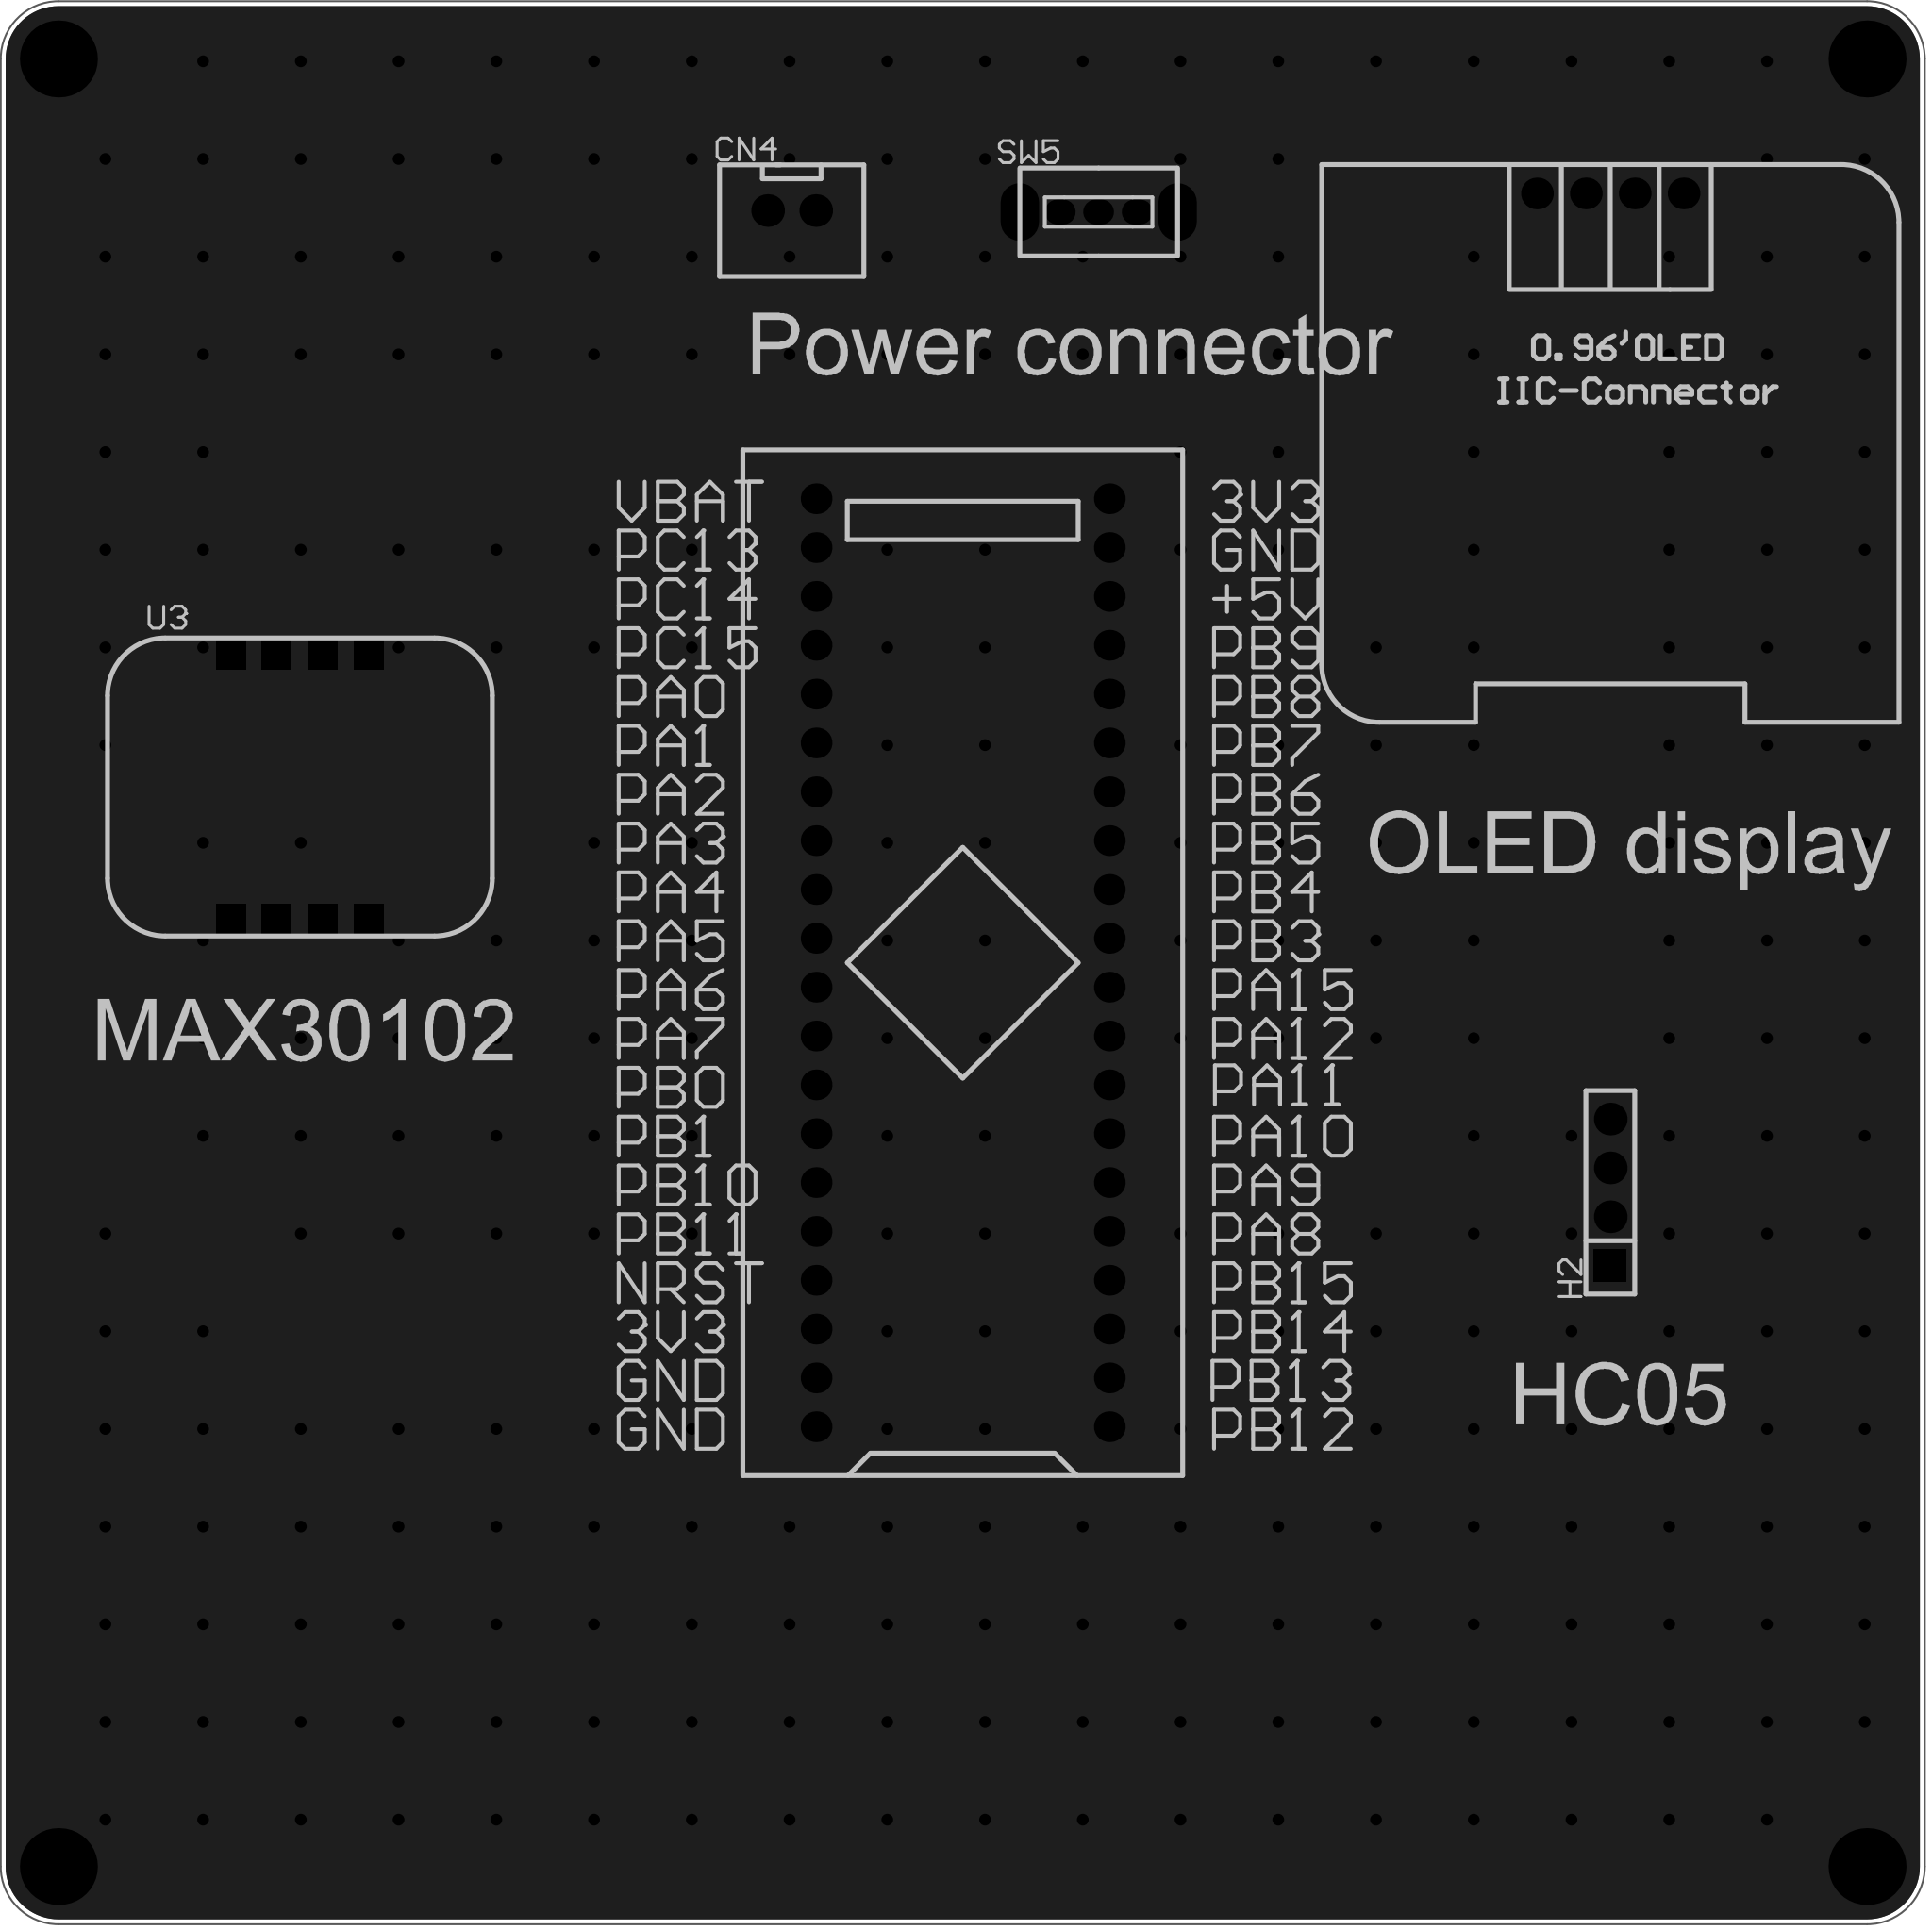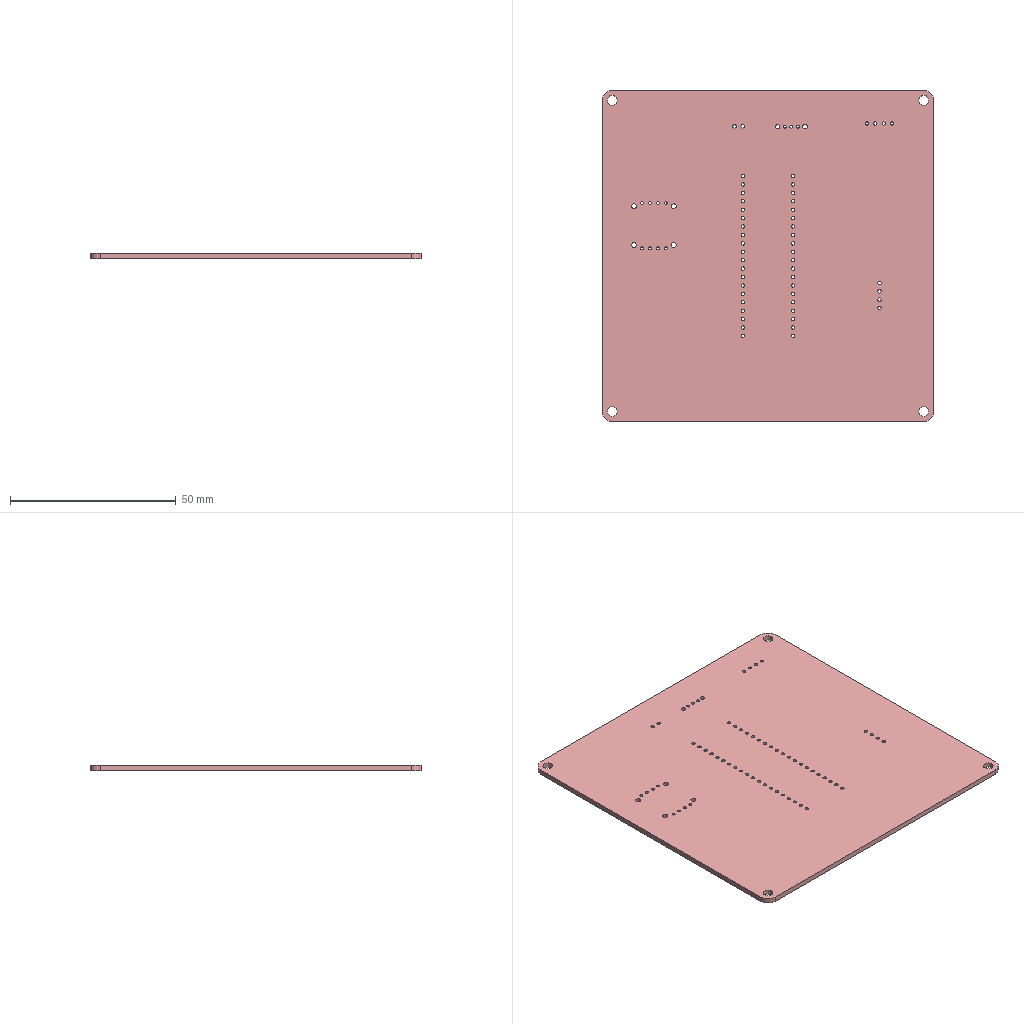Circuit board layout | Altium Designer | box 100 x 100 x 1.6 mm
Layer stack:
# Altium Designer layer stack of  (unit mm; dielectric type: 0 none, 1 core, 2 prepreg, 3 surface material)
index,name,kind,layer,copper_thickness_mm,dielectric_type,dielectric_thickness_mm,dielectric_material,dielectric_constant
0,Top Paste Mask Layer,other,,,,,,
1,Top Silkscreen Layer,other,,,,,,
2,Top Solder Mask Layer,dielectric,,,3,0.01,,3.3
3,Top Layer,copper,Top Layer,0.035,,,,
4,Dielectric1,dielectric,,,3,1.51,FR4,4.5
5,Bottom Layer,copper,Bottom Layer,0.035,,,,
6,Bottom Solder Mask Layer,dielectric,,,3,0.01,,3.3
7,Bottom Silkscreen Layer,other,,,,,,
8,Bottom Paste Mask Layer,other,,,,,,
# drill layer pairs: low layer,high layer
drill_pair,Top Layer,Bottom Layer
Part placement:
Designator,Comment,Layer,Footprint,Center-X(mm),Center-Y(mm),Rotation
U1,STM32F103C8T6-Card,TopLayer,CONN-TH_L53.3-W22.9_STM32F103C8T6-CARD,141.351,130.937,90
OLED1,,TopLayer,0.96OLED_4P,175.006,170.942,0
CN4,XH2.54*2P_THT,TopLayer,CONN-TH_2P-P2.50-XH2.54-2P,132.461,170.053,0
SW5,,TopLayer,拨动开关,148.417,169.978,0
H2,,TopLayer,HDR-TH_4P-P2.54-V-F,175.006,118.999,90
U3,MAX30102,TopLayer,MAX30102,106.901,140.081,0
Pad and via stacks:
# Altium Designer via and pad stacks of  (unit mm). Each distinct definition once, with the count of objects using it.
# via: kind,start_layer,end_layer,hole_mm,diameter_mm,mode(0 simple;1 top-mid-bottom;2 full stack),diameter_per_layer,count,example_net
# pad: kind,layer,hole_mm,hole_type(0 round;1 square;2 slot),plating,top_size,top_shape(1 round;2 rect;3 octagon;9 rounded rect),mid_size,bottom_size,mode,footprint,size_per_layer,count,example
pad,Multi-Layer,3,0,plated,4x4,1,4x4,4x4,0,,,4,1
pad,Multi-Layer,1,0,plated,1.6x1.6,1,1.6x1.6,1.6x1.6,0,CONN-TH_L53.3-W22.9_STM32F103C8T6-CARD,,40,U1.1
pad,Multi-Layer,1,0,plated,1.65x1.65,1,1.65x1.65,1.65x1.65,0,0.96OLED_4P,,4,OLED1.4
pad,Multi-Layer,1.05,0,plated,1.7x1.7,1,1.7x1.7,1.7x1.7,0,CONN-TH_2P-P2.50-XH2.54-2P,,2,CN4.2
pad,Multi-Layer,0.8992,0,plated,1.6x1.3,1,1.6x1.3,1.6x1.3,0,\u00B2\u00A6\u00B6\u00AF\u00BF\u00AA\u00B9\u00D8,,3,SW5.1
pad,Multi-Layer,1.3,0,plated,3x1.999,1,3x1.999,3x1.999,0,\u00B2\u00A6\u00B6\u00AF\u00BF\u00AA\u00B9\u00D8,,2,SW5.4
pad,Multi-Layer,1.1,0,plated,1.7x1.7,2,1.7x1.7,1.7x1.7,0,HDR-TH_4P-P2.54-V-F,,1,H2.1
pad,Multi-Layer,1.1,0,plated,1.7x1.7,1,1.7x1.7,1.7x1.7,0,HDR-TH_4P-P2.54-V-F,,3,H2.2
pad,Multi-Layer,0.9144,0,plated,1.524x1.524,2,1.524x1.524,1.524x1.524,0,MAX30102,,8,U3.1
via,Top Layer,Bottom Layer,0.3048,0.61,0,,286,GND
Copper pours:
name,layer,net,type(0 solid;1 hatched;2 none)
Bottom Layer-GND,Bottom Layer,GND,0
Top Layer-GND,Top Layer,GND,0